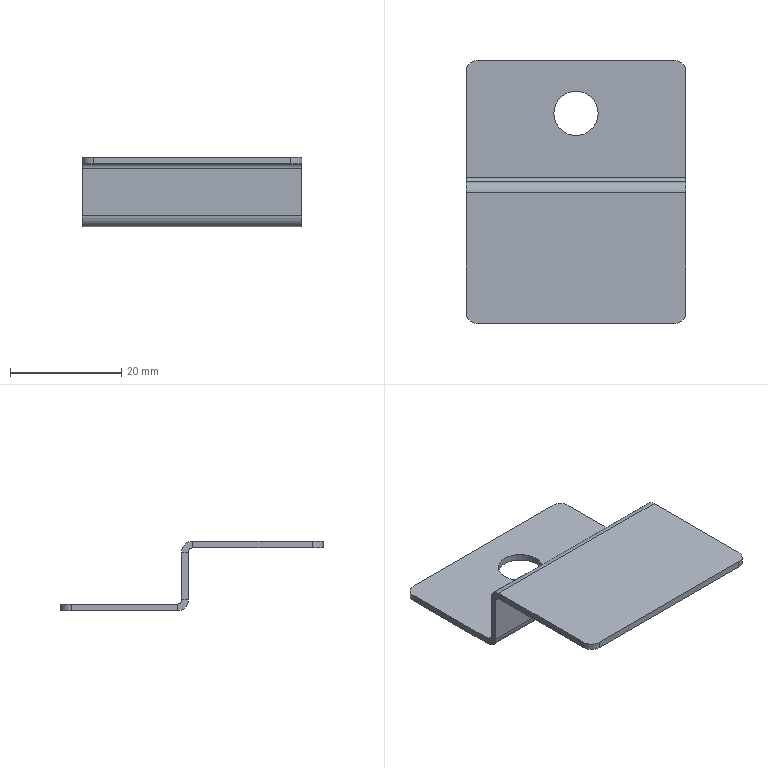Part | 1 solid | 28 faces | box 39.5 x 47.3 x 12.5 mm | volume 2659 mm3 | plane 18 | cylinder 10 | commonest cylinder face diameters 4 x4 1.48 x2 3.88 x2 8 x2
STEP:
#1=CARTESIAN_POINT('',(15.75,37.8,-12.5));
#2=VERTEX_POINT('',#1);
#3=CARTESIAN_POINT('',(23.75,37.8,-12.5));
#4=VERTEX_POINT('',#3);
#5=CARTESIAN_POINT('',(19.75,37.8,-12.5));
#6=DIRECTION('',(0.,0.,1.));
#7=DIRECTION('',(1.,0.,0.));
#8=AXIS2_PLACEMENT_3D('',#5,#6,#7);
#9=CIRCLE('',#8,4.);
#10=EDGE_CURVE('',#2,#4,#9,.T.);
#11=ORIENTED_EDGE('',*,*,#10,.F.);
#12=CARTESIAN_POINT('',(15.75,37.8,-11.3));
#13=VERTEX_POINT('',#12);
#14=CARTESIAN_POINT('',(15.75,37.8,-12.5));
#15=DIRECTION('',(0.,0.,1.));
#16=VECTOR('',#15,1000.);
#17=LINE('',#14,#16);
#18=EDGE_CURVE('',#2,#13,#17,.T.);
#19=ORIENTED_EDGE('',*,*,#18,.T.);
#20=CARTESIAN_POINT('',(23.75,37.8,-11.3));
#21=VERTEX_POINT('',#20);
#22=CARTESIAN_POINT('',(19.75,37.8,-11.3));
#23=DIRECTION('',(0.,0.,1.));
#24=DIRECTION('',(1.,0.,0.));
#25=AXIS2_PLACEMENT_3D('',#22,#23,#24);
#26=CIRCLE('',#25,4.);
#27=EDGE_CURVE('',#13,#21,#26,.T.);
#28=ORIENTED_EDGE('',*,*,#27,.T.);
#29=CARTESIAN_POINT('',(23.75,37.8,-12.5));
#30=DIRECTION('',(0.,0.,1.));
#31=VECTOR('',#30,1000.);
#32=LINE('',#29,#31);
#33=EDGE_CURVE('',#4,#21,#32,.T.);
#34=ORIENTED_EDGE('',*,*,#33,.F.);
#35=EDGE_LOOP('',(#11,#19,#28,#34));
#36=FACE_OUTER_BOUND('',#35,.T.);
#37=CARTESIAN_POINT('',(19.75,37.8,-12.5));
#38=DIRECTION('',(0.,0.,1.));
#39=DIRECTION('',(1.,0.,0.));
#40=AXIS2_PLACEMENT_3D('',#37,#38,#39);
#41=CYLINDRICAL_SURFACE('',#40,4.);
#42=ADVANCED_FACE('',(#36),#41,.F.);
#43=CARTESIAN_POINT('',(39.5,25.5,-10.56));
#44=VERTEX_POINT('',#43);
#45=CARTESIAN_POINT('',(39.5,24.3,-10.56));
#46=VERTEX_POINT('',#45);
#47=CARTESIAN_POINT('',(39.5,25.5,-10.56));
#48=DIRECTION('',(0.,-1.,0.));
#49=VECTOR('',#48,1000.);
#50=LINE('',#47,#49);
#51=EDGE_CURVE('',#44,#46,#50,.T.);
#52=ORIENTED_EDGE('',*,*,#51,.F.);
#53=CARTESIAN_POINT('',(39.5,25.5,-1.94));
#54=VERTEX_POINT('',#53);
#55=CARTESIAN_POINT('',(39.5,25.5,0.));
#56=DIRECTION('',(0.,0.,-1.));
#57=VECTOR('',#56,1000.);
#58=LINE('',#55,#57);
#59=EDGE_CURVE('',#54,#44,#58,.T.);
#60=ORIENTED_EDGE('',*,*,#59,.F.);
#61=CARTESIAN_POINT('',(39.5,24.3,-1.94));
#62=VERTEX_POINT('',#61);
#63=CARTESIAN_POINT('',(39.5,24.3,-1.94));
#64=DIRECTION('',(0.,1.,0.));
#65=VECTOR('',#64,1000.);
#66=LINE('',#63,#65);
#67=EDGE_CURVE('',#62,#54,#66,.T.);
#68=ORIENTED_EDGE('',*,*,#67,.F.);
#69=CARTESIAN_POINT('',(39.5,24.3,-12.5));
#70=DIRECTION('',(0.,0.,-1.));
#71=VECTOR('',#70,1000.);
#72=LINE('',#69,#71);
#73=EDGE_CURVE('',#62,#46,#72,.T.);
#74=ORIENTED_EDGE('',*,*,#73,.T.);
#75=EDGE_LOOP('',(#52,#60,#68,#74));
#76=FACE_OUTER_BOUND('',#75,.T.);
#77=CARTESIAN_POINT('',(39.5,25.5,-12.5));
#78=DIRECTION('',(-1.,0.,0.));
#79=DIRECTION('',(0.,0.,1.));
#80=AXIS2_PLACEMENT_3D('',#77,#78,#79);
#81=PLANE('',#80);
#82=ADVANCED_FACE('',(#76),#81,.F.);
#83=CARTESIAN_POINT('',(0.,25.5,-10.56));
#84=VERTEX_POINT('',#83);
#85=CARTESIAN_POINT('',(0.,24.3,-10.56));
#86=VERTEX_POINT('',#85);
#87=CARTESIAN_POINT('',(0.,25.5,-10.56));
#88=DIRECTION('',(0.,-1.,0.));
#89=VECTOR('',#88,1000.);
#90=LINE('',#87,#89);
#91=EDGE_CURVE('',#84,#86,#90,.T.);
#92=ORIENTED_EDGE('',*,*,#91,.T.);
#93=CARTESIAN_POINT('',(0.,24.3,-1.94));
#94=VERTEX_POINT('',#93);
#95=CARTESIAN_POINT('',(0.,24.3,-1.2));
#96=DIRECTION('',(0.,0.,1.));
#97=VECTOR('',#96,1000.);
#98=LINE('',#95,#97);
#99=EDGE_CURVE('',#86,#94,#98,.T.);
#100=ORIENTED_EDGE('',*,*,#99,.T.);
#101=CARTESIAN_POINT('',(0.,25.5,-1.94));
#102=VERTEX_POINT('',#101);
#103=CARTESIAN_POINT('',(0.,25.5,-1.94));
#104=DIRECTION('',(0.,1.,0.));
#105=VECTOR('',#104,1000.);
#106=LINE('',#103,#105);
#107=EDGE_CURVE('',#94,#102,#106,.T.);
#108=ORIENTED_EDGE('',*,*,#107,.T.);
#109=CARTESIAN_POINT('',(0.,25.5,0.));
#110=DIRECTION('',(0.,0.,1.));
#111=VECTOR('',#110,1000.);
#112=LINE('',#109,#111);
#113=EDGE_CURVE('',#84,#102,#112,.T.);
#114=ORIENTED_EDGE('',*,*,#113,.F.);
#115=EDGE_LOOP('',(#92,#100,#108,#114));
#116=FACE_OUTER_BOUND('',#115,.T.);
#117=CARTESIAN_POINT('',(0.,25.5,-1.2));
#118=DIRECTION('',(1.,0.,0.));
#119=DIRECTION('',(0.,0.,-1.));
#120=AXIS2_PLACEMENT_3D('',#117,#118,#119);
#121=PLANE('',#120);
#122=ADVANCED_FACE('',(#116),#121,.F.);
#123=CARTESIAN_POINT('',(0.,25.5,-10.56));
#124=DIRECTION('',(1.,0.,0.));
#125=VECTOR('',#124,1000.);
#126=LINE('',#123,#125);
#127=EDGE_CURVE('',#84,#44,#126,.T.);
#128=ORIENTED_EDGE('',*,*,#127,.F.);
#129=ORIENTED_EDGE('',*,*,#113,.T.);
#130=CARTESIAN_POINT('',(0.,25.5,-1.94));
#131=DIRECTION('',(-1.,0.,0.));
#132=VECTOR('',#131,1000.);
#133=LINE('',#130,#132);
#134=EDGE_CURVE('',#54,#102,#133,.T.);
#135=ORIENTED_EDGE('',*,*,#134,.F.);
#136=ORIENTED_EDGE('',*,*,#59,.T.);
#137=EDGE_LOOP('',(#128,#129,#135,#136));
#138=FACE_OUTER_BOUND('',#137,.T.);
#139=CARTESIAN_POINT('',(0.,25.5,0.));
#140=DIRECTION('',(0.,-1.,0.));
#141=DIRECTION('',(0.,0.,-1.));
#142=AXIS2_PLACEMENT_3D('',#139,#140,#141);
#143=PLANE('',#142);
#144=ADVANCED_FACE('',(#138),#143,.F.);
#145=ORIENTED_EDGE('',*,*,#99,.F.);
#146=CARTESIAN_POINT('',(0.,24.3,-10.56));
#147=DIRECTION('',(1.,0.,0.));
#148=VECTOR('',#147,1000.);
#149=LINE('',#146,#148);
#150=EDGE_CURVE('',#86,#46,#149,.T.);
#151=ORIENTED_EDGE('',*,*,#150,.T.);
#152=ORIENTED_EDGE('',*,*,#73,.F.);
#153=CARTESIAN_POINT('',(0.,24.3,-1.94));
#154=DIRECTION('',(1.,0.,0.));
#155=VECTOR('',#154,1000.);
#156=LINE('',#153,#155);
#157=EDGE_CURVE('',#94,#62,#156,.T.);
#158=ORIENTED_EDGE('',*,*,#157,.F.);
#159=EDGE_LOOP('',(#145,#151,#152,#158));
#160=FACE_OUTER_BOUND('',#159,.T.);
#161=CARTESIAN_POINT('',(0.,24.3,0.));
#162=DIRECTION('',(0.,-1.,0.));
#163=DIRECTION('',(0.,0.,-1.));
#164=AXIS2_PLACEMENT_3D('',#161,#162,#163);
#165=PLANE('',#164);
#166=ADVANCED_FACE('',(#160),#165,.T.);
#167=CARTESIAN_POINT('',(39.5,2.,0.));
#168=VERTEX_POINT('',#167);
#169=CARTESIAN_POINT('',(39.5,23.56,0.));
#170=VERTEX_POINT('',#169);
#171=CARTESIAN_POINT('',(39.5,0.,0.));
#172=DIRECTION('',(0.,1.,0.));
#173=VECTOR('',#172,1000.);
#174=LINE('',#171,#173);
#175=EDGE_CURVE('',#168,#170,#174,.T.);
#176=ORIENTED_EDGE('',*,*,#175,.F.);
#177=CARTESIAN_POINT('',(39.5,2.,-1.2));
#178=VERTEX_POINT('',#177);
#179=CARTESIAN_POINT('',(39.5,2.,-1.2));
#180=DIRECTION('',(0.,0.,-1.));
#181=VECTOR('',#180,1000.);
#182=LINE('',#179,#181);
#183=EDGE_CURVE('',#168,#178,#182,.T.);
#184=ORIENTED_EDGE('',*,*,#183,.T.);
#185=CARTESIAN_POINT('',(39.5,23.56,-1.2));
#186=VERTEX_POINT('',#185);
#187=CARTESIAN_POINT('',(39.5,0.,-1.2));
#188=DIRECTION('',(0.,1.,0.));
#189=VECTOR('',#188,1000.);
#190=LINE('',#187,#189);
#191=EDGE_CURVE('',#178,#186,#190,.T.);
#192=ORIENTED_EDGE('',*,*,#191,.T.);
#193=CARTESIAN_POINT('',(39.5,23.56,-1.2));
#194=DIRECTION('',(0.,0.,1.));
#195=VECTOR('',#194,1000.);
#196=LINE('',#193,#195);
#197=EDGE_CURVE('',#186,#170,#196,.T.);
#198=ORIENTED_EDGE('',*,*,#197,.T.);
#199=EDGE_LOOP('',(#176,#184,#192,#198));
#200=FACE_OUTER_BOUND('',#199,.T.);
#201=CARTESIAN_POINT('',(39.5,0.,-1.2));
#202=DIRECTION('',(1.,0.,0.));
#203=DIRECTION('',(0.,0.,-1.));
#204=AXIS2_PLACEMENT_3D('',#201,#202,#203);
#205=PLANE('',#204);
#206=ADVANCED_FACE('',(#200),#205,.T.);
#207=ORIENTED_EDGE('',*,*,#191,.F.);
#208=CARTESIAN_POINT('',(37.5,0.,-1.2));
#209=VERTEX_POINT('',#208);
#210=CARTESIAN_POINT('',(37.5,2.,-1.2));
#211=DIRECTION('',(0.,0.,-1.));
#212=DIRECTION('',(-1.,0.,0.));
#213=AXIS2_PLACEMENT_3D('',#210,#211,#212);
#214=CIRCLE('',#213,2.);
#215=EDGE_CURVE('',#178,#209,#214,.T.);
#216=ORIENTED_EDGE('',*,*,#215,.T.);
#217=CARTESIAN_POINT('',(2.,0.,-1.2));
#218=VERTEX_POINT('',#217);
#219=CARTESIAN_POINT('',(0.,0.,-1.2));
#220=DIRECTION('',(1.,0.,0.));
#221=VECTOR('',#220,1000.);
#222=LINE('',#219,#221);
#223=EDGE_CURVE('',#218,#209,#222,.T.);
#224=ORIENTED_EDGE('',*,*,#223,.F.);
#225=CARTESIAN_POINT('',(0.,2.,-1.2));
#226=VERTEX_POINT('',#225);
#227=CARTESIAN_POINT('',(2.,2.,-1.2));
#228=DIRECTION('',(0.,0.,-1.));
#229=DIRECTION('',(-1.,0.,0.));
#230=AXIS2_PLACEMENT_3D('',#227,#228,#229);
#231=CIRCLE('',#230,2.);
#232=EDGE_CURVE('',#218,#226,#231,.T.);
#233=ORIENTED_EDGE('',*,*,#232,.T.);
#234=CARTESIAN_POINT('',(0.,23.56,-1.2));
#235=VERTEX_POINT('',#234);
#236=CARTESIAN_POINT('',(0.,0.,-1.2));
#237=DIRECTION('',(0.,-1.,0.));
#238=VECTOR('',#237,1000.);
#239=LINE('',#236,#238);
#240=EDGE_CURVE('',#235,#226,#239,.T.);
#241=ORIENTED_EDGE('',*,*,#240,.F.);
#242=CARTESIAN_POINT('',(39.5,23.56,-1.2));
#243=DIRECTION('',(-1.,0.,0.));
#244=VECTOR('',#243,1000.);
#245=LINE('',#242,#244);
#246=EDGE_CURVE('',#186,#235,#245,.T.);
#247=ORIENTED_EDGE('',*,*,#246,.F.);
#248=EDGE_LOOP('',(#207,#216,#224,#233,#241,#247));
#249=FACE_OUTER_BOUND('',#248,.T.);
#250=CARTESIAN_POINT('',(0.,0.,-1.2));
#251=DIRECTION('',(0.,0.,-1.));
#252=DIRECTION('',(-1.,0.,0.));
#253=AXIS2_PLACEMENT_3D('',#250,#251,#252);
#254=PLANE('',#253);
#255=ADVANCED_FACE('',(#249),#254,.T.);
#256=CARTESIAN_POINT('',(2.,0.,0.));
#257=VERTEX_POINT('',#256);
#258=CARTESIAN_POINT('',(37.5,0.,0.));
#259=VERTEX_POINT('',#258);
#260=CARTESIAN_POINT('',(0.,0.,0.));
#261=DIRECTION('',(1.,0.,0.));
#262=VECTOR('',#261,1000.);
#263=LINE('',#260,#262);
#264=EDGE_CURVE('',#257,#259,#263,.T.);
#265=ORIENTED_EDGE('',*,*,#264,.T.);
#266=CARTESIAN_POINT('',(37.5,2.,0.));
#267=DIRECTION('',(0.,0.,1.));
#268=DIRECTION('',(-1.,0.,0.));
#269=AXIS2_PLACEMENT_3D('',#266,#267,#268);
#270=CIRCLE('',#269,2.);
#271=EDGE_CURVE('',#259,#168,#270,.T.);
#272=ORIENTED_EDGE('',*,*,#271,.T.);
#273=ORIENTED_EDGE('',*,*,#175,.T.);
#274=CARTESIAN_POINT('',(0.,23.56,0.));
#275=VERTEX_POINT('',#274);
#276=CARTESIAN_POINT('',(39.5,23.56,0.));
#277=DIRECTION('',(-1.,0.,0.));
#278=VECTOR('',#277,1000.);
#279=LINE('',#276,#278);
#280=EDGE_CURVE('',#170,#275,#279,.T.);
#281=ORIENTED_EDGE('',*,*,#280,.T.);
#282=CARTESIAN_POINT('',(0.,2.,0.));
#283=VERTEX_POINT('',#282);
#284=CARTESIAN_POINT('',(0.,0.,0.));
#285=DIRECTION('',(0.,-1.,0.));
#286=VECTOR('',#285,1000.);
#287=LINE('',#284,#286);
#288=EDGE_CURVE('',#275,#283,#287,.T.);
#289=ORIENTED_EDGE('',*,*,#288,.T.);
#290=CARTESIAN_POINT('',(2.,2.,0.));
#291=DIRECTION('',(0.,0.,1.));
#292=DIRECTION('',(-1.,0.,0.));
#293=AXIS2_PLACEMENT_3D('',#290,#291,#292);
#294=CIRCLE('',#293,2.);
#295=EDGE_CURVE('',#283,#257,#294,.T.);
#296=ORIENTED_EDGE('',*,*,#295,.T.);
#297=EDGE_LOOP('',(#265,#272,#273,#281,#289,#296));
#298=FACE_OUTER_BOUND('',#297,.T.);
#299=CARTESIAN_POINT('',(0.,0.,0.));
#300=DIRECTION('',(0.,0.,-1.));
#301=DIRECTION('',(-1.,0.,0.));
#302=AXIS2_PLACEMENT_3D('',#299,#300,#301);
#303=PLANE('',#302);
#304=ADVANCED_FACE('',(#298),#303,.F.);
#305=ORIENTED_EDGE('',*,*,#240,.T.);
#306=CARTESIAN_POINT('',(0.,2.,-1.2));
#307=DIRECTION('',(0.,0.,1.));
#308=VECTOR('',#307,1000.);
#309=LINE('',#306,#308);
#310=EDGE_CURVE('',#226,#283,#309,.T.);
#311=ORIENTED_EDGE('',*,*,#310,.T.);
#312=ORIENTED_EDGE('',*,*,#288,.F.);
#313=CARTESIAN_POINT('',(0.,23.56,-1.2));
#314=DIRECTION('',(0.,0.,1.));
#315=VECTOR('',#314,1000.);
#316=LINE('',#313,#315);
#317=EDGE_CURVE('',#235,#275,#316,.T.);
#318=ORIENTED_EDGE('',*,*,#317,.F.);
#319=EDGE_LOOP('',(#305,#311,#312,#318));
#320=FACE_OUTER_BOUND('',#319,.T.);
#321=CARTESIAN_POINT('',(0.,0.,-1.2));
#322=DIRECTION('',(-1.,0.,0.));
#323=DIRECTION('',(0.,0.,1.));
#324=AXIS2_PLACEMENT_3D('',#321,#322,#323);
#325=PLANE('',#324);
#326=ADVANCED_FACE('',(#320),#325,.T.);
#327=ORIENTED_EDGE('',*,*,#223,.T.);
#328=CARTESIAN_POINT('',(37.5,0.,-1.2));
#329=DIRECTION('',(0.,0.,1.));
#330=VECTOR('',#329,1000.);
#331=LINE('',#328,#330);
#332=EDGE_CURVE('',#209,#259,#331,.T.);
#333=ORIENTED_EDGE('',*,*,#332,.T.);
#334=ORIENTED_EDGE('',*,*,#264,.F.);
#335=CARTESIAN_POINT('',(2.,0.,-1.2));
#336=DIRECTION('',(0.,0.,-1.));
#337=VECTOR('',#336,1000.);
#338=LINE('',#335,#337);
#339=EDGE_CURVE('',#257,#218,#338,.T.);
#340=ORIENTED_EDGE('',*,*,#339,.T.);
#341=EDGE_LOOP('',(#327,#333,#334,#340));
#342=FACE_OUTER_BOUND('',#341,.T.);
#343=CARTESIAN_POINT('',(0.,0.,-1.2));
#344=DIRECTION('',(0.,-1.,0.));
#345=DIRECTION('',(0.,0.,-1.));
#346=AXIS2_PLACEMENT_3D('',#343,#344,#345);
#347=PLANE('',#346);
#348=ADVANCED_FACE('',(#342),#347,.T.);
#349=ORIENTED_EDGE('',*,*,#107,.F.);
#350=CARTESIAN_POINT('',(0.,23.56,-1.94));
#351=DIRECTION('',(-1.,0.,0.));
#352=DIRECTION('',(0.,0.,-1.));
#353=AXIS2_PLACEMENT_3D('',#350,#351,#352);
#354=CIRCLE('',#353,0.74);
#355=EDGE_CURVE('',#235,#94,#354,.T.);
#356=ORIENTED_EDGE('',*,*,#355,.F.);
#357=ORIENTED_EDGE('',*,*,#317,.T.);
#358=CARTESIAN_POINT('',(0.,23.56,-1.94));
#359=DIRECTION('',(-1.,0.,0.));
#360=DIRECTION('',(0.,0.,-1.));
#361=AXIS2_PLACEMENT_3D('',#358,#359,#360);
#362=CIRCLE('',#361,1.94);
#363=EDGE_CURVE('',#275,#102,#362,.T.);
#364=ORIENTED_EDGE('',*,*,#363,.T.);
#365=EDGE_LOOP('',(#349,#356,#357,#364));
#366=FACE_OUTER_BOUND('',#365,.T.);
#367=CARTESIAN_POINT('',(0.,23.56,-1.94));
#368=DIRECTION('',(-1.,0.,0.));
#369=DIRECTION('',(0.,0.,1.));
#370=AXIS2_PLACEMENT_3D('',#367,#368,#369);
#371=PLANE('',#370);
#372=ADVANCED_FACE('',(#366),#371,.T.);
#373=CARTESIAN_POINT('',(39.5,23.56,-1.94));
#374=DIRECTION('',(1.,0.,0.));
#375=DIRECTION('',(0.,0.,-1.));
#376=AXIS2_PLACEMENT_3D('',#373,#374,#375);
#377=CIRCLE('',#376,0.74);
#378=EDGE_CURVE('',#62,#186,#377,.T.);
#379=ORIENTED_EDGE('',*,*,#378,.F.);
#380=ORIENTED_EDGE('',*,*,#67,.T.);
#381=CARTESIAN_POINT('',(39.5,23.56,-1.94));
#382=DIRECTION('',(1.,0.,0.));
#383=DIRECTION('',(0.,0.,-1.));
#384=AXIS2_PLACEMENT_3D('',#381,#382,#383);
#385=CIRCLE('',#384,1.94);
#386=EDGE_CURVE('',#54,#170,#385,.T.);
#387=ORIENTED_EDGE('',*,*,#386,.T.);
#388=ORIENTED_EDGE('',*,*,#197,.F.);
#389=EDGE_LOOP('',(#379,#380,#387,#388));
#390=FACE_OUTER_BOUND('',#389,.T.);
#391=CARTESIAN_POINT('',(39.5,23.56,-1.94));
#392=DIRECTION('',(-1.,0.,0.));
#393=DIRECTION('',(0.,0.,1.));
#394=AXIS2_PLACEMENT_3D('',#391,#392,#393);
#395=PLANE('',#394);
#396=ADVANCED_FACE('',(#390),#395,.F.);
#397=ORIENTED_EDGE('',*,*,#280,.F.);
#398=ORIENTED_EDGE('',*,*,#386,.F.);
#399=ORIENTED_EDGE('',*,*,#134,.T.);
#400=ORIENTED_EDGE('',*,*,#363,.F.);
#401=EDGE_LOOP('',(#397,#398,#399,#400));
#402=FACE_OUTER_BOUND('',#401,.T.);
#403=CARTESIAN_POINT('',(39.5,23.56,-1.94));
#404=DIRECTION('',(1.,0.,0.));
#405=DIRECTION('',(0.,1.,0.));
#406=AXIS2_PLACEMENT_3D('',#403,#404,#405);
#407=CYLINDRICAL_SURFACE('',#406,1.94);
#408=ADVANCED_FACE('',(#402),#407,.T.);
#409=ORIENTED_EDGE('',*,*,#246,.T.);
#410=ORIENTED_EDGE('',*,*,#355,.T.);
#411=ORIENTED_EDGE('',*,*,#157,.T.);
#412=ORIENTED_EDGE('',*,*,#378,.T.);
#413=EDGE_LOOP('',(#409,#410,#411,#412));
#414=FACE_OUTER_BOUND('',#413,.T.);
#415=CARTESIAN_POINT('',(39.5,23.56,-1.94));
#416=DIRECTION('',(1.,0.,0.));
#417=DIRECTION('',(0.,1.,0.));
#418=AXIS2_PLACEMENT_3D('',#415,#416,#417);
#419=CYLINDRICAL_SURFACE('',#418,0.74);
#420=ADVANCED_FACE('',(#414),#419,.F.);
#421=CARTESIAN_POINT('',(39.5,26.24,-11.3));
#422=VERTEX_POINT('',#421);
#423=CARTESIAN_POINT('',(39.5,26.24,-12.5));
#424=VERTEX_POINT('',#423);
#425=CARTESIAN_POINT('',(39.5,26.24,-12.5));
#426=DIRECTION('',(0.,0.,-1.));
#427=VECTOR('',#426,1000.);
#428=LINE('',#425,#427);
#429=EDGE_CURVE('',#422,#424,#428,.T.);
#430=ORIENTED_EDGE('',*,*,#429,.F.);
#431=CARTESIAN_POINT('',(39.5,26.24,-10.56));
#432=DIRECTION('',(1.,0.,0.));
#433=DIRECTION('',(0.,-1.,0.));
#434=AXIS2_PLACEMENT_3D('',#431,#432,#433);
#435=CIRCLE('',#434,0.74);
#436=EDGE_CURVE('',#44,#422,#435,.T.);
#437=ORIENTED_EDGE('',*,*,#436,.F.);
#438=ORIENTED_EDGE('',*,*,#51,.T.);
#439=CARTESIAN_POINT('',(39.5,26.24,-10.56));
#440=DIRECTION('',(1.,0.,0.));
#441=DIRECTION('',(0.,-1.,0.));
#442=AXIS2_PLACEMENT_3D('',#439,#440,#441);
#443=CIRCLE('',#442,1.94);
#444=EDGE_CURVE('',#46,#424,#443,.T.);
#445=ORIENTED_EDGE('',*,*,#444,.T.);
#446=EDGE_LOOP('',(#430,#437,#438,#445));
#447=FACE_OUTER_BOUND('',#446,.T.);
#448=CARTESIAN_POINT('',(39.5,26.24,-10.56));
#449=DIRECTION('',(1.,0.,0.));
#450=DIRECTION('',(0.,1.,0.));
#451=AXIS2_PLACEMENT_3D('',#448,#449,#450);
#452=PLANE('',#451);
#453=ADVANCED_FACE('',(#447),#452,.T.);
#454=CARTESIAN_POINT('',(0.,26.24,-11.3));
#455=VERTEX_POINT('',#454);
#456=CARTESIAN_POINT('',(0.,26.24,-10.56));
#457=DIRECTION('',(-1.,0.,0.));
#458=DIRECTION('',(0.,-1.,0.));
#459=AXIS2_PLACEMENT_3D('',#456,#457,#458);
#460=CIRCLE('',#459,0.74);
#461=EDGE_CURVE('',#455,#84,#460,.T.);
#462=ORIENTED_EDGE('',*,*,#461,.F.);
#463=CARTESIAN_POINT('',(0.,26.24,-12.5));
#464=VERTEX_POINT('',#463);
#465=CARTESIAN_POINT('',(0.,26.24,-11.3));
#466=DIRECTION('',(0.,0.,-1.));
#467=VECTOR('',#466,1000.);
#468=LINE('',#465,#467);
#469=EDGE_CURVE('',#455,#464,#468,.T.);
#470=ORIENTED_EDGE('',*,*,#469,.T.);
#471=CARTESIAN_POINT('',(0.,26.24,-10.56));
#472=DIRECTION('',(-1.,0.,0.));
#473=DIRECTION('',(0.,-1.,0.));
#474=AXIS2_PLACEMENT_3D('',#471,#472,#473);
#475=CIRCLE('',#474,1.94);
#476=EDGE_CURVE('',#464,#86,#475,.T.);
#477=ORIENTED_EDGE('',*,*,#476,.T.);
#478=ORIENTED_EDGE('',*,*,#91,.F.);
#479=EDGE_LOOP('',(#462,#470,#477,#478));
#480=FACE_OUTER_BOUND('',#479,.T.);
#481=CARTESIAN_POINT('',(0.,26.24,-10.56));
#482=DIRECTION('',(1.,0.,0.));
#483=DIRECTION('',(0.,1.,0.));
#484=AXIS2_PLACEMENT_3D('',#481,#482,#483);
#485=PLANE('',#484);
#486=ADVANCED_FACE('',(#480),#485,.F.);
#487=ORIENTED_EDGE('',*,*,#150,.F.);
#488=ORIENTED_EDGE('',*,*,#476,.F.);
#489=CARTESIAN_POINT('',(0.,26.24,-12.5));
#490=DIRECTION('',(-1.,0.,0.));
#491=VECTOR('',#490,1000.);
#492=LINE('',#489,#491);
#493=EDGE_CURVE('',#424,#464,#492,.T.);
#494=ORIENTED_EDGE('',*,*,#493,.F.);
#495=ORIENTED_EDGE('',*,*,#444,.F.);
#496=EDGE_LOOP('',(#487,#488,#494,#495));
#497=FACE_OUTER_BOUND('',#496,.T.);
#498=CARTESIAN_POINT('',(0.,26.24,-10.56));
#499=DIRECTION('',(-1.,0.,0.));
#500=DIRECTION('',(0.,0.,-1.));
#501=AXIS2_PLACEMENT_3D('',#498,#499,#500);
#502=CYLINDRICAL_SURFACE('',#501,1.94);
#503=ADVANCED_FACE('',(#497),#502,.T.);
#504=ORIENTED_EDGE('',*,*,#127,.T.);
#505=ORIENTED_EDGE('',*,*,#436,.T.);
#506=CARTESIAN_POINT('',(39.5,26.24,-11.3));
#507=DIRECTION('',(-1.,0.,0.));
#508=VECTOR('',#507,1000.);
#509=LINE('',#506,#508);
#510=EDGE_CURVE('',#422,#455,#509,.T.);
#511=ORIENTED_EDGE('',*,*,#510,.T.);
#512=ORIENTED_EDGE('',*,*,#461,.T.);
#513=EDGE_LOOP('',(#504,#505,#511,#512));
#514=FACE_OUTER_BOUND('',#513,.T.);
#515=CARTESIAN_POINT('',(0.,26.24,-10.56));
#516=DIRECTION('',(-1.,0.,0.));
#517=DIRECTION('',(0.,0.,-1.));
#518=AXIS2_PLACEMENT_3D('',#515,#516,#517);
#519=CYLINDRICAL_SURFACE('',#518,0.74);
#520=ADVANCED_FACE('',(#514),#519,.F.);
#521=CARTESIAN_POINT('',(0.,45.3,-11.3));
#522=VERTEX_POINT('',#521);
#523=CARTESIAN_POINT('',(0.,0.,-11.3));
#524=DIRECTION('',(0.,-1.,0.));
#525=VECTOR('',#524,1000.);
#526=LINE('',#523,#525);
#527=EDGE_CURVE('',#522,#455,#526,.T.);
#528=ORIENTED_EDGE('',*,*,#527,.F.);
#529=CARTESIAN_POINT('',(0.,45.3,-12.5));
#530=VERTEX_POINT('',#529);
#531=CARTESIAN_POINT('',(0.,45.3,-12.5));
#532=DIRECTION('',(0.,0.,-1.));
#533=VECTOR('',#532,1000.);
#534=LINE('',#531,#533);
#535=EDGE_CURVE('',#522,#530,#534,.T.);
#536=ORIENTED_EDGE('',*,*,#535,.T.);
#537=CARTESIAN_POINT('',(0.,25.5,-12.5));
#538=DIRECTION('',(0.,-1.,0.));
#539=VECTOR('',#538,1000.);
#540=LINE('',#537,#539);
#541=EDGE_CURVE('',#530,#464,#540,.T.);
#542=ORIENTED_EDGE('',*,*,#541,.T.);
#543=ORIENTED_EDGE('',*,*,#469,.F.);
#544=EDGE_LOOP('',(#528,#536,#542,#543));
#545=FACE_OUTER_BOUND('',#544,.T.);
#546=CARTESIAN_POINT('',(0.,25.5,-12.5));
#547=DIRECTION('',(-1.,0.,0.));
#548=DIRECTION('',(0.,0.,1.));
#549=AXIS2_PLACEMENT_3D('',#546,#547,#548);
#550=PLANE('',#549);
#551=ADVANCED_FACE('',(#545),#550,.T.);
#552=CARTESIAN_POINT('',(39.5,45.3,-12.5));
#553=VERTEX_POINT('',#552);
#554=CARTESIAN_POINT('',(39.5,47.3,-12.5));
#555=DIRECTION('',(0.,1.,0.));
#556=VECTOR('',#555,1000.);
#557=LINE('',#554,#556);
#558=EDGE_CURVE('',#424,#553,#557,.T.);
#559=ORIENTED_EDGE('',*,*,#558,.T.);
#560=CARTESIAN_POINT('',(39.5,45.3,-11.3));
#561=VERTEX_POINT('',#560);
#562=CARTESIAN_POINT('',(39.5,45.3,-12.5));
#563=DIRECTION('',(0.,0.,1.));
#564=VECTOR('',#563,1000.);
#565=LINE('',#562,#564);
#566=EDGE_CURVE('',#553,#561,#565,.T.);
#567=ORIENTED_EDGE('',*,*,#566,.T.);
#568=CARTESIAN_POINT('',(39.5,0.,-11.3));
#569=DIRECTION('',(0.,1.,0.));
#570=VECTOR('',#569,1000.);
#571=LINE('',#568,#570);
#572=EDGE_CURVE('',#422,#561,#571,.T.);
#573=ORIENTED_EDGE('',*,*,#572,.F.);
#574=ORIENTED_EDGE('',*,*,#429,.T.);
#575=EDGE_LOOP('',(#559,#567,#573,#574));
#576=FACE_OUTER_BOUND('',#575,.T.);
#577=CARTESIAN_POINT('',(39.5,47.3,-12.5));
#578=DIRECTION('',(1.,0.,0.));
#579=DIRECTION('',(0.,0.,-1.));
#580=AXIS2_PLACEMENT_3D('',#577,#578,#579);
#581=PLANE('',#580);
#582=ADVANCED_FACE('',(#576),#581,.T.);
#583=CARTESIAN_POINT('',(19.75,37.8,-12.5));
#584=DIRECTION('',(0.,0.,1.));
#585=DIRECTION('',(1.,0.,0.));
#586=AXIS2_PLACEMENT_3D('',#583,#584,#585);
#587=CIRCLE('',#586,4.);
#588=EDGE_CURVE('',#4,#2,#587,.T.);
#589=ORIENTED_EDGE('',*,*,#588,.T.);
#590=ORIENTED_EDGE('',*,*,#10,.T.);
#591=EDGE_LOOP('',(#589,#590));
#592=FACE_BOUND('',#591,.T.);
#593=ORIENTED_EDGE('',*,*,#541,.F.);
#594=CARTESIAN_POINT('',(2.,47.3,-12.5));
#595=VERTEX_POINT('',#594);
#596=CARTESIAN_POINT('',(2.,45.3,-12.5));
#597=DIRECTION('',(0.,0.,-1.));
#598=DIRECTION('',(-1.,0.,0.));
#599=AXIS2_PLACEMENT_3D('',#596,#597,#598);
#600=CIRCLE('',#599,2.);
#601=EDGE_CURVE('',#530,#595,#600,.T.);
#602=ORIENTED_EDGE('',*,*,#601,.T.);
#603=CARTESIAN_POINT('',(37.5,47.3,-12.5));
#604=VERTEX_POINT('',#603);
#605=CARTESIAN_POINT('',(0.,47.3,-12.5));
#606=DIRECTION('',(-1.,0.,0.));
#607=VECTOR('',#606,1000.);
#608=LINE('',#605,#607);
#609=EDGE_CURVE('',#604,#595,#608,.T.);
#610=ORIENTED_EDGE('',*,*,#609,.F.);
#611=CARTESIAN_POINT('',(37.5,45.3,-12.5));
#612=DIRECTION('',(0.,0.,-1.));
#613=DIRECTION('',(-1.,0.,0.));
#614=AXIS2_PLACEMENT_3D('',#611,#612,#613);
#615=CIRCLE('',#614,2.);
#616=EDGE_CURVE('',#604,#553,#615,.T.);
#617=ORIENTED_EDGE('',*,*,#616,.T.);
#618=ORIENTED_EDGE('',*,*,#558,.F.);
#619=ORIENTED_EDGE('',*,*,#493,.T.);
#620=EDGE_LOOP('',(#593,#602,#610,#617,#618,#619));
#621=FACE_OUTER_BOUND('',#620,.T.);
#622=CARTESIAN_POINT('',(0.,0.,-12.5));
#623=DIRECTION('',(0.,0.,-1.));
#624=DIRECTION('',(-1.,0.,0.));
#625=AXIS2_PLACEMENT_3D('',#622,#623,#624);
#626=PLANE('',#625);
#627=ADVANCED_FACE('',(#592,#621),#626,.T.);
#628=CARTESIAN_POINT('',(19.75,37.8,-11.3));
#629=DIRECTION('',(0.,0.,1.));
#630=DIRECTION('',(1.,0.,0.));
#631=AXIS2_PLACEMENT_3D('',#628,#629,#630);
#632=CIRCLE('',#631,4.);
#633=EDGE_CURVE('',#21,#13,#632,.T.);
#634=ORIENTED_EDGE('',*,*,#633,.F.);
#635=ORIENTED_EDGE('',*,*,#27,.F.);
#636=EDGE_LOOP('',(#634,#635));
#637=FACE_BOUND('',#636,.T.);
#638=CARTESIAN_POINT('',(37.5,47.3,-11.3));
#639=VERTEX_POINT('',#638);
#640=CARTESIAN_POINT('',(2.,47.3,-11.3));
#641=VERTEX_POINT('',#640);
#642=CARTESIAN_POINT('',(0.,47.3,-11.3));
#643=DIRECTION('',(-1.,0.,0.));
#644=VECTOR('',#643,1000.);
#645=LINE('',#642,#644);
#646=EDGE_CURVE('',#639,#641,#645,.T.);
#647=ORIENTED_EDGE('',*,*,#646,.T.);
#648=CARTESIAN_POINT('',(2.,45.3,-11.3));
#649=DIRECTION('',(0.,0.,1.));
#650=DIRECTION('',(-1.,0.,0.));
#651=AXIS2_PLACEMENT_3D('',#648,#649,#650);
#652=CIRCLE('',#651,2.);
#653=EDGE_CURVE('',#641,#522,#652,.T.);
#654=ORIENTED_EDGE('',*,*,#653,.T.);
#655=ORIENTED_EDGE('',*,*,#527,.T.);
#656=ORIENTED_EDGE('',*,*,#510,.F.);
#657=ORIENTED_EDGE('',*,*,#572,.T.);
#658=CARTESIAN_POINT('',(37.5,45.3,-11.3));
#659=DIRECTION('',(0.,0.,1.));
#660=DIRECTION('',(-1.,0.,0.));
#661=AXIS2_PLACEMENT_3D('',#658,#659,#660);
#662=CIRCLE('',#661,2.);
#663=EDGE_CURVE('',#561,#639,#662,.T.);
#664=ORIENTED_EDGE('',*,*,#663,.T.);
#665=EDGE_LOOP('',(#647,#654,#655,#656,#657,#664));
#666=FACE_OUTER_BOUND('',#665,.T.);
#667=CARTESIAN_POINT('',(0.,0.,-11.3));
#668=DIRECTION('',(0.,0.,-1.));
#669=DIRECTION('',(-1.,0.,0.));
#670=AXIS2_PLACEMENT_3D('',#667,#668,#669);
#671=PLANE('',#670);
#672=ADVANCED_FACE('',(#637,#666),#671,.F.);
#673=ORIENTED_EDGE('',*,*,#609,.T.);
#674=CARTESIAN_POINT('',(2.,47.3,-12.5));
#675=DIRECTION('',(0.,0.,1.));
#676=VECTOR('',#675,1000.);
#677=LINE('',#674,#676);
#678=EDGE_CURVE('',#595,#641,#677,.T.);
#679=ORIENTED_EDGE('',*,*,#678,.T.);
#680=ORIENTED_EDGE('',*,*,#646,.F.);
#681=CARTESIAN_POINT('',(37.5,47.3,-12.5));
#682=DIRECTION('',(0.,0.,-1.));
#683=VECTOR('',#682,1000.);
#684=LINE('',#681,#683);
#685=EDGE_CURVE('',#639,#604,#684,.T.);
#686=ORIENTED_EDGE('',*,*,#685,.T.);
#687=EDGE_LOOP('',(#673,#679,#680,#686));
#688=FACE_OUTER_BOUND('',#687,.T.);
#689=CARTESIAN_POINT('',(0.,47.3,-12.5));
#690=DIRECTION('',(0.,1.,0.));
#691=DIRECTION('',(0.,0.,1.));
#692=AXIS2_PLACEMENT_3D('',#689,#690,#691);
#693=PLANE('',#692);
#694=ADVANCED_FACE('',(#688),#693,.T.);
#695=ORIENTED_EDGE('',*,*,#18,.F.);
#696=ORIENTED_EDGE('',*,*,#588,.F.);
#697=ORIENTED_EDGE('',*,*,#33,.T.);
#698=ORIENTED_EDGE('',*,*,#633,.T.);
#699=EDGE_LOOP('',(#695,#696,#697,#698));
#700=FACE_OUTER_BOUND('',#699,.T.);
#701=CARTESIAN_POINT('',(19.75,37.8,-12.5));
#702=DIRECTION('',(0.,0.,1.));
#703=DIRECTION('',(1.,0.,0.));
#704=AXIS2_PLACEMENT_3D('',#701,#702,#703);
#705=CYLINDRICAL_SURFACE('',#704,4.);
#706=ADVANCED_FACE('',(#700),#705,.F.);
#707=ORIENTED_EDGE('',*,*,#215,.F.);
#708=ORIENTED_EDGE('',*,*,#183,.F.);
#709=ORIENTED_EDGE('',*,*,#271,.F.);
#710=ORIENTED_EDGE('',*,*,#332,.F.);
#711=EDGE_LOOP('',(#707,#708,#709,#710));
#712=FACE_OUTER_BOUND('',#711,.T.);
#713=CARTESIAN_POINT('',(37.5,2.,-1.2));
#714=DIRECTION('',(0.,0.,1.));
#715=DIRECTION('',(1.,0.,0.));
#716=AXIS2_PLACEMENT_3D('',#713,#714,#715);
#717=CYLINDRICAL_SURFACE('',#716,2.);
#718=ADVANCED_FACE('',(#712),#717,.T.);
#719=ORIENTED_EDGE('',*,*,#232,.F.);
#720=ORIENTED_EDGE('',*,*,#339,.F.);
#721=ORIENTED_EDGE('',*,*,#295,.F.);
#722=ORIENTED_EDGE('',*,*,#310,.F.);
#723=EDGE_LOOP('',(#719,#720,#721,#722));
#724=FACE_OUTER_BOUND('',#723,.T.);
#725=CARTESIAN_POINT('',(2.,2.,-1.2));
#726=DIRECTION('',(0.,0.,1.));
#727=DIRECTION('',(1.,0.,0.));
#728=AXIS2_PLACEMENT_3D('',#725,#726,#727);
#729=CYLINDRICAL_SURFACE('',#728,2.);
#730=ADVANCED_FACE('',(#724),#729,.T.);
#731=ORIENTED_EDGE('',*,*,#601,.F.);
#732=ORIENTED_EDGE('',*,*,#535,.F.);
#733=ORIENTED_EDGE('',*,*,#653,.F.);
#734=ORIENTED_EDGE('',*,*,#678,.F.);
#735=EDGE_LOOP('',(#731,#732,#733,#734));
#736=FACE_OUTER_BOUND('',#735,.T.);
#737=CARTESIAN_POINT('',(2.,45.3,-12.5));
#738=DIRECTION('',(0.,0.,1.));
#739=DIRECTION('',(1.,0.,0.));
#740=AXIS2_PLACEMENT_3D('',#737,#738,#739);
#741=CYLINDRICAL_SURFACE('',#740,2.);
#742=ADVANCED_FACE('',(#736),#741,.T.);
#743=ORIENTED_EDGE('',*,*,#616,.F.);
#744=ORIENTED_EDGE('',*,*,#685,.F.);
#745=ORIENTED_EDGE('',*,*,#663,.F.);
#746=ORIENTED_EDGE('',*,*,#566,.F.);
#747=EDGE_LOOP('',(#743,#744,#745,#746));
#748=FACE_OUTER_BOUND('',#747,.T.);
#749=CARTESIAN_POINT('',(37.5,45.3,-12.5));
#750=DIRECTION('',(0.,0.,1.));
#751=DIRECTION('',(1.,0.,0.));
#752=AXIS2_PLACEMENT_3D('',#749,#750,#751);
#753=CYLINDRICAL_SURFACE('',#752,2.);
#754=ADVANCED_FACE('',(#748),#753,.T.);
#755=CLOSED_SHELL('',(#42,#82,#122,#144,#166,#206,#255,#304,#326,#348,#372,#396,#408,#420,#453,#486,#503,#520,#551,#582,#627,#672,#694,#706,#718,#730,#742,#754));
#756=MANIFOLD_SOLID_BREP('',#755);
#757=CARTESIAN_POINT('',(0.,0.,0.));
#758=DIRECTION('',(0.,0.,1.));
#759=DIRECTION('',(1.,0.,0.));
#760=AXIS2_PLACEMENT_3D('',#757,#758,#759);
#761=(LENGTH_UNIT()NAMED_UNIT(*)SI_UNIT(.MILLI.,.METRE.));
#762=UNCERTAINTY_MEASURE_WITH_UNIT(LENGTH_MEASURE(0.00001),#761,'','');
#763=(NAMED_UNIT(*)PLANE_ANGLE_UNIT()SI_UNIT($,.RADIAN.));
#764=(NAMED_UNIT(*)SI_UNIT($,.STERADIAN.)SOLID_ANGLE_UNIT());
#765=(GEOMETRIC_REPRESENTATION_CONTEXT(3)GLOBAL_UNCERTAINTY_ASSIGNED_CONTEXT((#762))GLOBAL_UNIT_ASSIGNED_CONTEXT((#761,#763,#764))REPRESENTATION_CONTEXT('',''));
#766=ADVANCED_BREP_SHAPE_REPRESENTATION('',(#756,#760),#765);